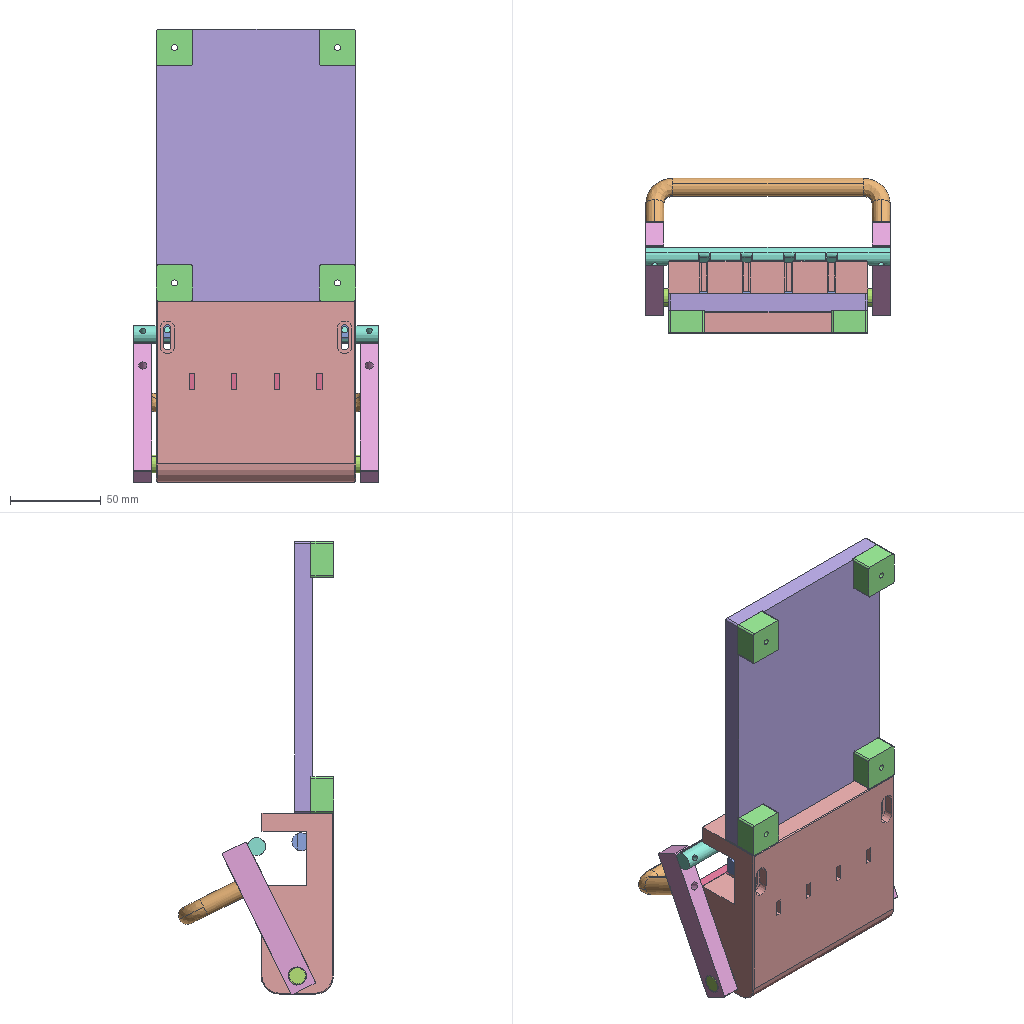Assembly | SolidWorks | 9 different items | 13 placed | box 135 x 86 x 250 mm
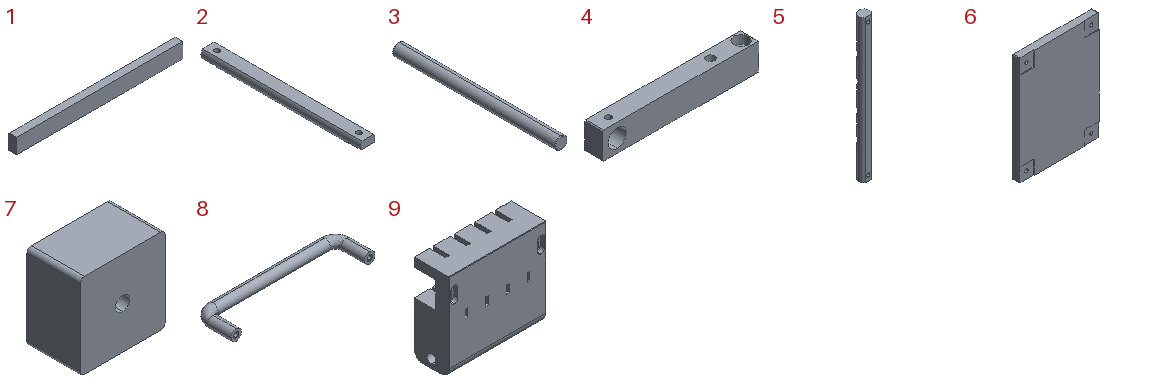Parts list (item | quantity | size | volume | features):
1 | x1 | 110 x 5 x 10 mm | 5325 mm3 | features Extrusion 1, ICE 1
2 | x1 | 10 x 110 x 8 mm | 6927 mm3 | features ICE 2, Extrusion 1, HoleWzd 1, MirrorPattern 1
3 | x1 | 10 x 135 x 10 mm | 10600 mm3 | features Extrusion 1, Fillet 1
4 | x2 | 87 x 10 x 15 mm | 11602 mm3 | features HoleWzd 3, Chamfer 1, Extrusion 1, ICE 1
5 | x1 | 10 x 9 x 135 mm | 9423 mm3 | features ICE 3, Chamfer 1, Extrusion 1, Fillet 1, HoleWzd 1
6 | x1 | 110 x 10 x 150 mm | 162821 mm3 | features Fillet 2, Extrusion 1, HoleWzd 1, ICE 1
7 | x4 | 20 x 12.5 x 20 mm | 4882 mm3 | features Extrusion 1, Fillet 1, HoleWzd 1
8 | x1 | 135 x 37 x 10 mm | 13834 mm3 | features MBimport 1
9 | x1 | 110 x 40 x 100 mm | 333751 mm3 | features ICE 7, Chamfer 3, Extrusion 1, Fillet 1, HoleWzd 1
Mates (type | each side: item.copy, entity, surface, feature):
Concentric | 9.1 face cylinder Cut-Extrude6 | 3.1 face cylinder Boss-Extrude1
Concentric | 3.1 face cylinder Boss-Extrude1 | 4.1 face cylinder Cut-Extrude1
Coincident | 3.1 face plane Boss-Extrude1 | 4.1 face plane Boss-Extrude1
Coincident | 9.1 face plane Cut-Extrude5 | 2.1 face plane Cut-Extrude1
Concentric | 3.1 face cylinder Boss-Extrude1 | 4.2 face cylinder Cut-Extrude1
Coincident | 4.1 face plane Boss-Extrude1 | 5.1 face plane Cut-Extrude1
Coincident | 4.2 face plane Boss-Extrude1 | 5.1 face plane Cut-Extrude1
Concentric | 4.2 face cylinder CBORE for M4 Slotted cheese head screws2 | 5.1 face cylinder M4 Tapped Hole1
Concentric | 4.1 face cylinder CBORE for M4 Slotted cheese head screws2 | 5.1 face cylinder M4 Tapped Hole1
Concentric | 4.1 face cylinder Ø4.5 (4.5) Diameter Hole2 | 8.1 face cylinder E-LUWANS10-125-27.STEP<1>
Concentric | 4.2 face cylinder Ø4.5 (4.5) Diameter Hole2 | 8.1 face cylinder E-LUWANS10-125-27.STEP<1>
Coincident | 4.2 face plane Boss-Extrude1 | 8.1 face plane E-LUWANS10-125-27.STEP<1>
Width | 2.1 face plane Boss-Extrude1 | 2.1 face plane Boss-Extrude1 | 9.1 face plane Boss-Extrude2 | 9.1 face plane Boss-Extrude2
Coincident | 9.1 face plane Boss-Extrude2 | 6.1 face plane Boss-Extrude1 | 2 times
Coincident | 6.1 face plane Cut-Extrude1 | 7.1 face plane Boss-Extrude1 | 2 times
Concentric | 6.1 face cylinder Ø4.5 (4.5) Diameter Hole1 | 7.1 face cylinder M4 Tapped Hole1
Coincident | 9.1 face plane Boss-Extrude2 | 7.1 face plane Boss-Extrude1
Coincident | 6.1 face plane Cut-Extrude1 | 7.2 face plane Boss-Extrude1 | 2 times
Concentric | 6.1 face cylinder Ø4.5 (4.5) Diameter Hole1 | 7.2 face cylinder M4 Tapped Hole1
Coincident | 6.1 face plane Cut-Extrude1 | 7.3 face plane Boss-Extrude1 | 2 times
Concentric | 6.1 face cylinder Ø4.5 (4.5) Diameter Hole1 | 7.3 face cylinder M4 Tapped Hole1
Coincident | 6.1 face plane Cut-Extrude1 | 7.4 face plane Boss-Extrude1 | 2 times
Concentric | 6.1 face cylinder Ø4.5 (4.5) Diameter Hole1 | 7.4 face cylinder M4 Tapped Hole1
Concentric | 9.1 face cylinder Cut-Extrude10 | 1.1 face cylinder Cut-Extrude1 | 2 times
Coincident | 9.1 face plane Boss-Extrude2 | 1.1 face plane Boss-Extrude1
Width | 3.1 face plane Boss-Extrude1 | 3.1 face plane Boss-Extrude1 | 9.1 face plane Boss-Extrude2 | 9.1 face plane Boss-Extrude2